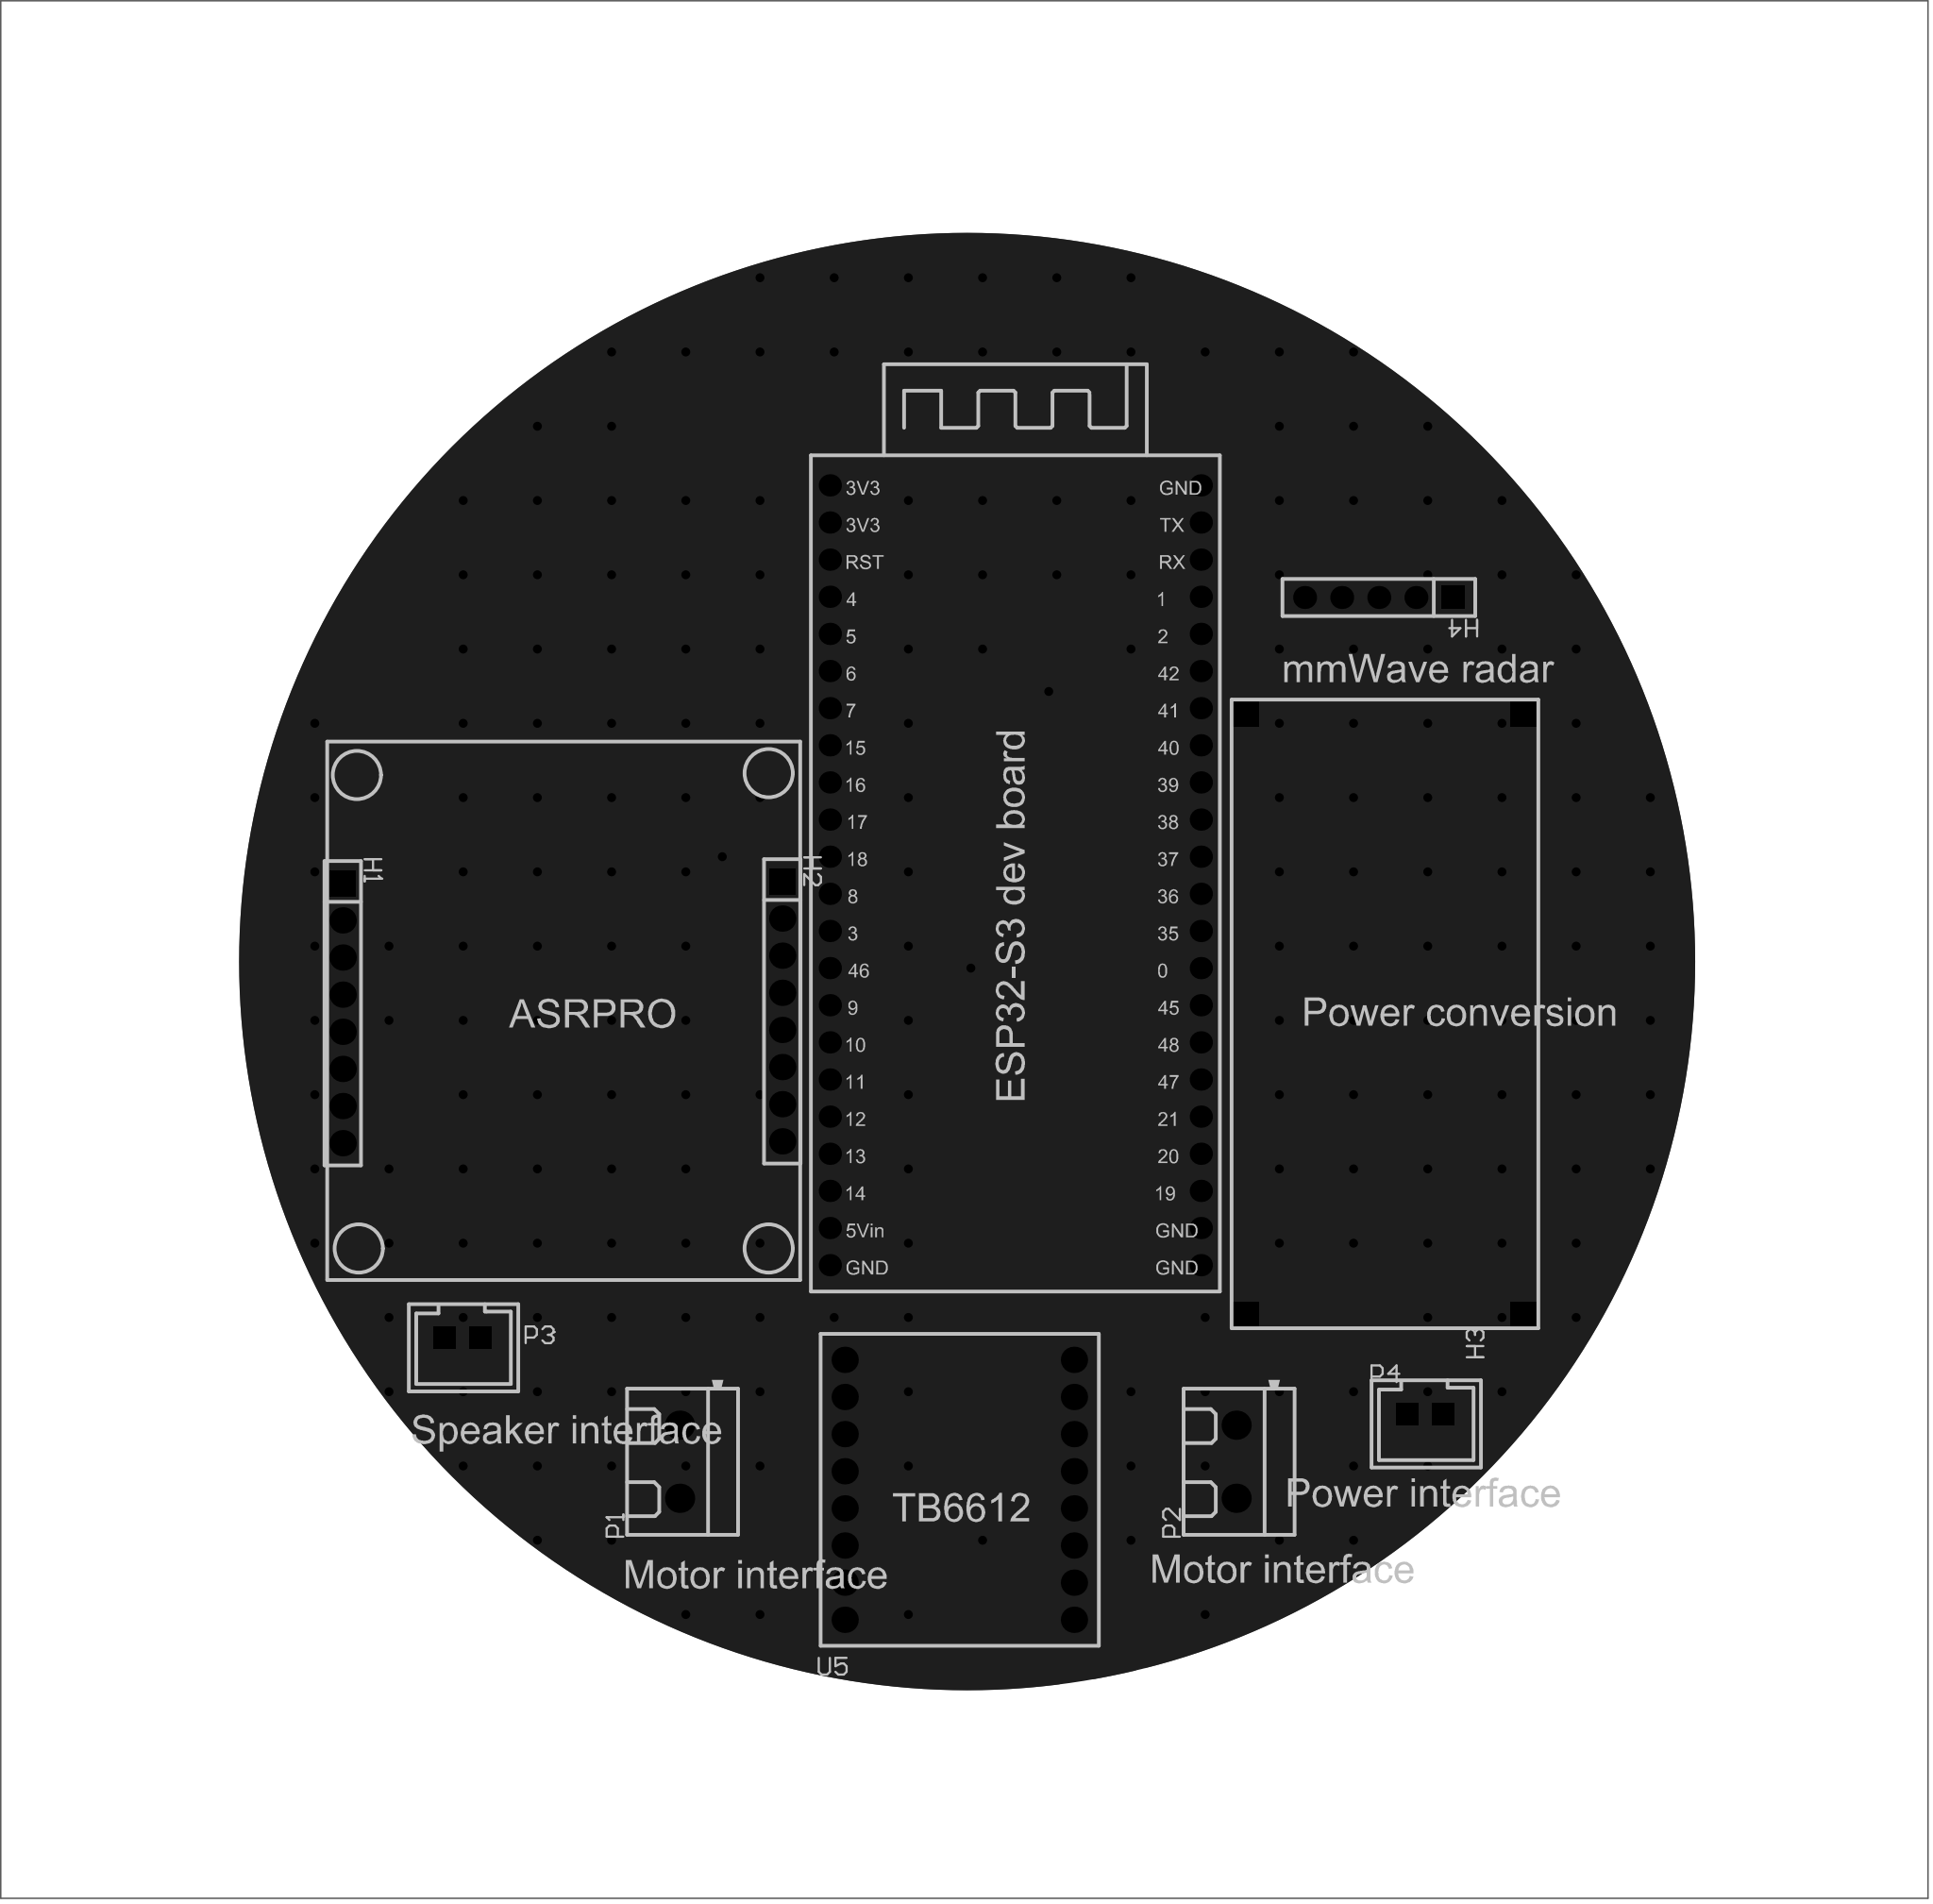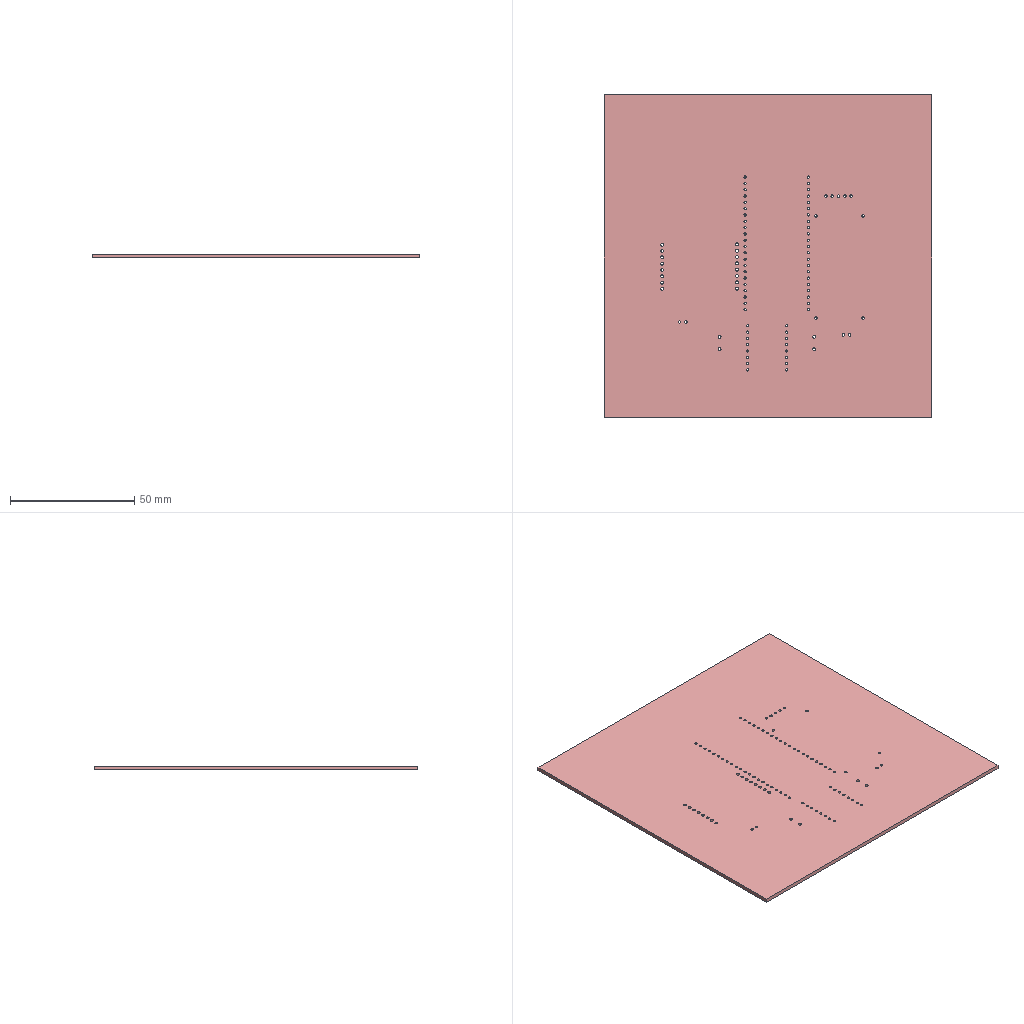Circuit board layout | Altium Designer | box 132 x 129.8 x 1.6 mm
Layer stack:
# Altium Designer layer stack of  (unit mm; dielectric type: 0 none, 1 core, 2 prepreg, 3 surface material)
index,name,kind,layer,copper_thickness_mm,dielectric_type,dielectric_thickness_mm,dielectric_material,dielectric_constant
0,Top Paste Mask Layer,other,,,,,,
1,Top Silkscreen Layer,other,,,,,,
2,Top Solder Mask Layer,dielectric,,,3,0.01,,3.3
3,Top Layer,copper,Top Layer,0.035,,,,
4,Dielectric1,dielectric,,,3,1.51,FR4,4.5
5,Bottom Layer,copper,Bottom Layer,0.035,,,,
6,Bottom Solder Mask Layer,dielectric,,,3,0.01,,3.3
7,Bottom Silkscreen Layer,other,,,,,,
8,Bottom Paste Mask Layer,other,,,,,,
# drill layer pairs: low layer,high layer
drill_pair,Top Layer,Bottom Layer
Part placement:
Designator,Comment,Layer,Footprint,Center-X(mm),Center-Y(mm),Rotation
U4,NO,TopLayer,ESP32S3,139.319,139.827,0
P1,KF301-2P terminal block,TopLayer,CONN-TH_XY301V-A-5.0-2P,116.332,99.711,90
P2,KF301-2P terminal block,TopLayer,CONN-TH_XY301V-A-5.0-2P,154.436,99.711,90
U5,,TopLayer,tb6612,135.484,97.79,0
H1,,TopLayer,HDR-TH_8P-P2.54-V-F-1,93.265,130.391,270
H2,,TopLayer,HDR-TH_8P-P2.54-V-F-1,123.359,130.518,270
H3,,TopLayer,HDR-TH_4P-P2.54-V-F-R2-C2-S2.54,164.617,130.315,90
P3,XH2.54 straight socket-2P,TopLayer,CONN-TH_XH2.54-2P,101.473,108.204,180
P4,XH2.54 straight socket-2P,TopLayer,CONN-TH_XH2.54-2P,167.386,102.997,180
H4,,TopLayer,HDR-TH_5P-P2.54-V-F,164.204,158.827,180
Pad and via stacks:
# Altium Designer via and pad stacks of  (unit mm). Each distinct definition once, with the count of objects using it.
# via: kind,start_layer,end_layer,hole_mm,diameter_mm,mode(0 simple;1 top-mid-bottom;2 full stack),diameter_per_layer,count,example_net
# pad: kind,layer,hole_mm,hole_type(0 round;1 square;2 slot),plating,top_size,top_shape(1 round;2 rect;3 octagon;9 rounded rect),mid_size,bottom_size,mode,footprint,size_per_layer,count,example
pad,Multi-Layer,0.9144,0,plated,1.524x1.524,1,1.524x1.524,1.524x1.524,0,ESP32S3,,44,U4.1
pad,Multi-Layer,1.2,0,plated,2x2,1,2x2,2x2,0,CONN-TH_XY301V-A-5.0-2P,,4,P1.1
pad,Multi-Layer,0.9,0,plated,1.8x1.8,1,1.8x1.8,1.8x1.8,0,tb6612,,16,U5.1
pad,Multi-Layer,1.2,0,plated,1.8x1.8,2,1.8x1.8,1.8x1.8,0,HDR-TH_8P-P2.54-V-F-1,,2,H1.1
pad,Multi-Layer,1.2,0,plated,1.8x1.8,1,1.8x1.8,1.8x1.8,0,HDR-TH_8P-P2.54-V-F-1,,14,H1.2
pad,Multi-Layer,1,0,plated,1.8x1.8,2,1.8x1.8,1.8x1.8,0,HDR-TH_4P-P2.54-V-F-R2-C2-S2.54,,4,H3.2
pad,Multi-Layer,1,2,plated,1.524x1.524,2,1.524x1.524,1.524x1.524,0,CONN-TH_XH2.54-2P,,4,P3.1
pad,Multi-Layer,1.02,0,plated,1.575x1.575,1,1.575x1.575,1.575x1.575,0,HDR-TH_5P-P2.54-V-F,,4,H4.5
pad,Multi-Layer,1.02,0,plated,1.575x1.575,2,1.575x1.575,1.575x1.575,0,HDR-TH_5P-P2.54-V-F,,1,H4.1
via,Top Layer,Bottom Layer,0.3048,0.61,0,,3,1
via,Top Layer,Bottom Layer,0.3048,0.6096,0,,208,GND
Copper pours:
name,layer,net,type(0 solid;1 hatched;2 none)
Top Layer-GND,Top Layer,GND,0
Bottom Layer-GND,Bottom Layer,GND,0
Design rules, without the lines most boards share:
# Altium Designer design rules of  (exported by Altium Designer, unit mm)
# columns: name | kind | enabled | priority | scope1 | scope2 | descriptor | typed fields (field=value)
Plane_Default | 0 | disabled | 1 | All | All | Clearance Constraint (Gap=6mil) (Disabled)(All),(All) | gap=0.1524
Plane_Default_1 | 63 | disabled | 1 | All | All | Board Clearance Constraint (Gap=0mil) (Disabled)(All) |
Copper_Default | 0 | disabled | 2 | All | All | Clearance Constraint (Gap=6mil) (Disabled)(All),(All) | gap=0.1524
Copper_Default_1 | 63 | disabled | 2 | All | All | Board Clearance Constraint (Gap=0mil) (Disabled)(All) |
Copper_gge24019 | 0 | disabled | 3 | All | All | Clearance Constraint (Gap=6mil) (Disabled)(All),(All) | gap=0.1524
Copper_gge24019_1 | 63 | disabled | 3 | All | All | Board Clearance Constraint (Gap=0mil) (Disabled)(All) |
Default | 0 | enabled | 4 | All | All | Clearance Constraint (Gap=6mil) (All),(All) | gap=0.1524
Default_1 | 63 | enabled | 4 | All | All | Board Clearance Constraint (Gap=0mil) (All) |
otherClearance | 52 | enabled | 1 | All | All | Hole To Hole Clearance (Gap=11.8mil) (All),(All) | gap=0.2997
Default_2 | 2 | enabled | 1 | All | All | Width Constraint (Min=10mil) (Max=1000mil) (Preferred=10mil) (All) |
Default_3 | 11 | enabled | 1 | All | All | Routing Via (MinHoleWidth=12mil) (MaxHoleWidth=2362mil) (PreferredHoleWidth=12mil) (MinWidth=24mil) (MaxWidth=3938mil) (PreferedWidth=24mil) (All) | via_min_hole=0.3048 via_max_hole=59.995 via_preferred_diameter=0.6096 via_preferred_hole=0.3048
Default_4 | 6 | enabled | 1 | All | All | Power Plane Connect Rule(Relief Connect )(Expansion=20mil) (Conductor Width=0mil) (Air Gap=10mil) (Entries=4) (All) | relief_conductor_width=0 relief_entries=4 relief_expansion=0.508
gge24019 | 20 | disabled | 1 | All | All | Polygon Connect Rule(Relief Connect )(Conductor Width=0mil) (Relief Angle=90 Angle) (Entries=4) (Air Gap Width=1mil) (Disabled)(All),(All) | connect_style(0=relief,1=direct,2=none)=0 relief_conductor_width=0 relief_entries=4
Default_5 | 20 | enabled | 2 | All | All | Polygon Connect Rule(Relief Connect )(Conductor Width=0mil) (Relief Angle=90 Angle) (Entries=4) (Air Gap Width=1mil) (All),(All) | connect_style(0=relief,1=direct,2=none)=0 relief_conductor_width=0 relief_entries=4
Common | 14 | enabled | 1 | All | All | Paste Mask Expansion (Expansion =0mil) (All) | expansion=0
Common_1 | 13 | enabled | 2 | All | All | Solder Mask Expansion (Expansion =2mil) (All) | expansion=0.0508
Common_2 | 13 | enabled | 1 | IsVia | All | Solder Mask Expansion (Expansion =-1000mil) (IsVia) | expansion=-25.4